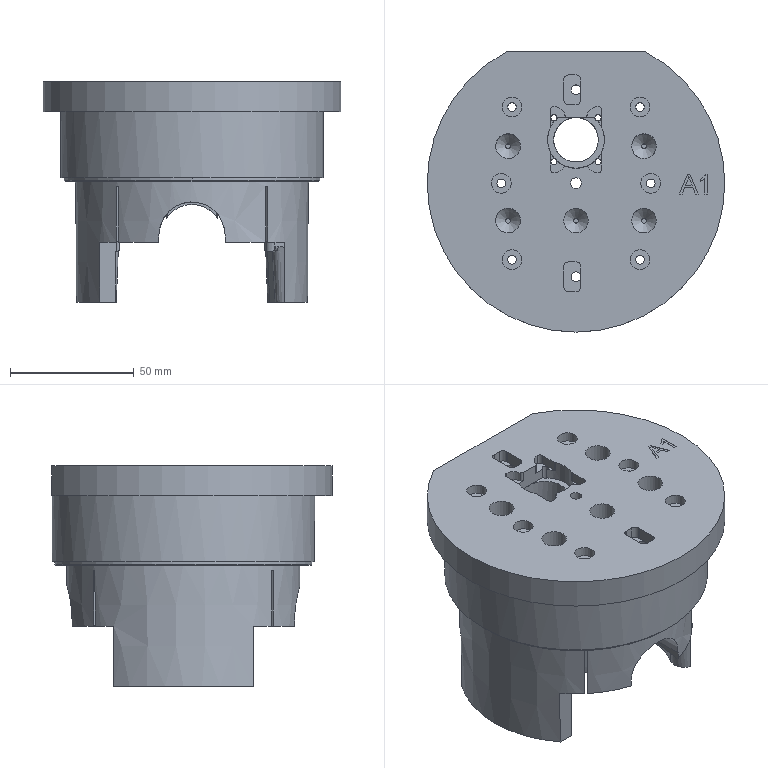Part | NX | features solid 2 | 1 solid | 273 faces | box 120 x 113.014 x 88.91 mm | volume 472884 mm3 | plane 97 | cylinder 84 | spline 47 | torus 21 | cone 14 | sphere 10 | commonest cylinder face diameters 4 x10 2 x8 3.5 x6 8 x6 10 x5 24.622 x5